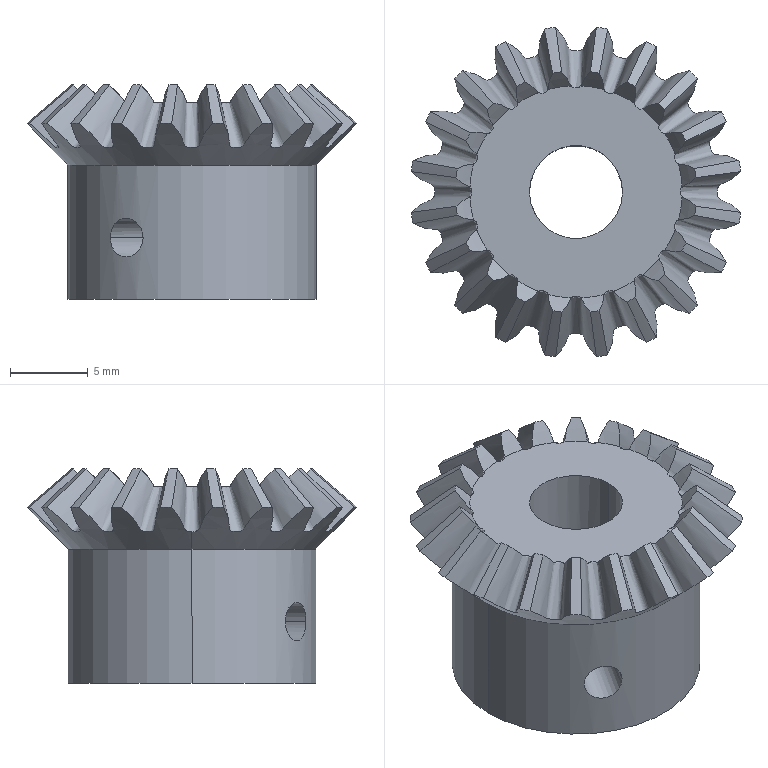Part | SolidWorks | features 3DProfileFeature 9, ICE 2, BlendCut 1, CirPattern 1, CurveInFile 1, HoleWzd 1, RefAxis 1, RevCut 1, Revolution 1 | 1 solid | 75 faces | box 21.253 x 21.253 x 13.804 mm | volume 2380 mm3 | cone 44 | spline 20 | cylinder 9 | plane 2 | commonest cylinder face diameters 2.5 x5 6 x2 16 x2